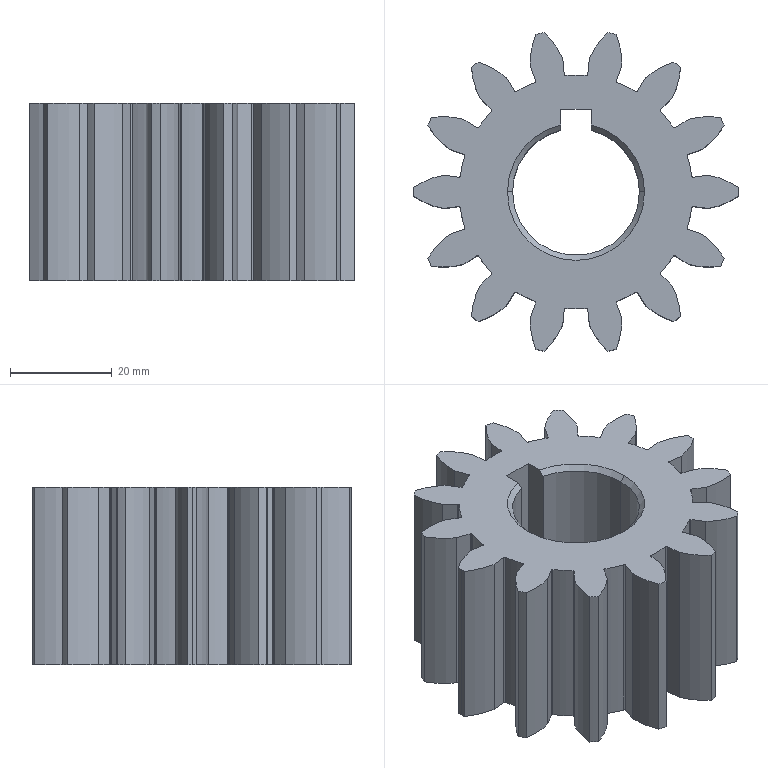Part | SolidWorks | features BaseBody 1, Chamfer 1, Fillet 1, ICE 1, RevCut 1 | 1 solid | 133 faces | box 64 x 62.751 x 35 mm | volume 62928 mm3 | cylinder 66 | plane 33 | spline 28 | cone 6 | commonest cylinder face diameters 0.6 x34 64 x15 46 x14 25 x3